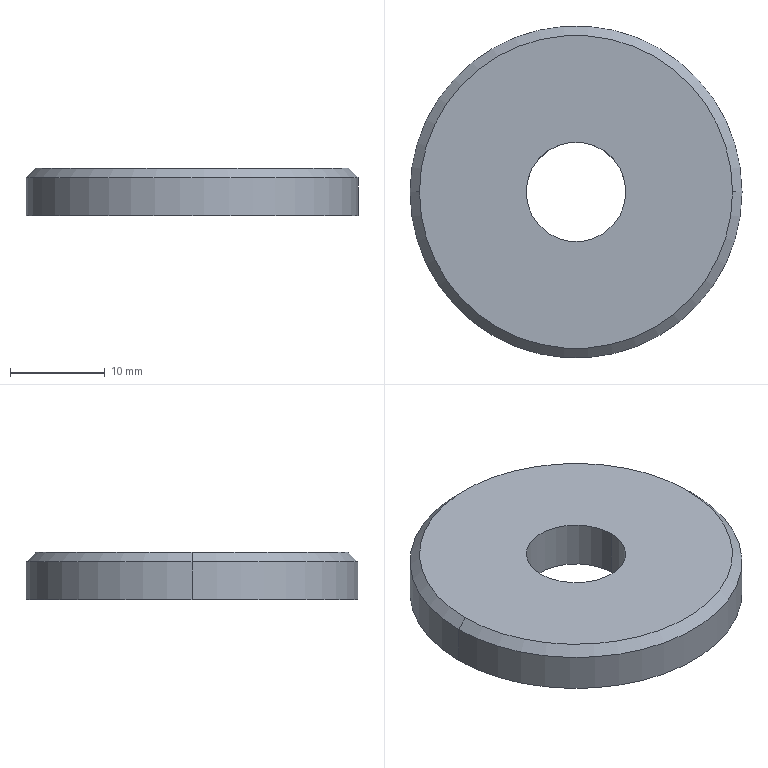Part | SolidWorks | features Chamfer 1, Extrusion 1 | 1 solid | 8 faces | box 35 x 35 x 5 mm | volume 4324 mm3 | cylinder 4 | cone 2 | plane 2 | commonest cylinder face diameters 10.5 x2 35 x2
STEP:
#1=CARTESIAN_POINT('',(16.5,0.,5.));
#2=VERTEX_POINT('',#1);
#3=CARTESIAN_POINT('',(-16.5,0.,5.));
#4=VERTEX_POINT('',#3);
#5=CARTESIAN_POINT('',(0.,0.,5.));
#6=DIRECTION('',(0.,0.,1.));
#7=DIRECTION('',(1.,0.,0.));
#8=AXIS2_PLACEMENT_3D('',#5,#6,#7);
#9=CIRCLE('',#8,16.5);
#10=EDGE_CURVE('',#2,#4,#9,.T.);
#11=ORIENTED_EDGE('',*,*,#10,.F.);
#12=CARTESIAN_POINT('',(17.5,0.,4.));
#13=VERTEX_POINT('',#12);
#14=CARTESIAN_POINT('',(16.5,0.,5.));
#15=DIRECTION('',(0.7071,0.,-0.7071));
#16=VECTOR('',#15,1000.);
#17=LINE('',#14,#16);
#18=EDGE_CURVE('',#2,#13,#17,.T.);
#19=ORIENTED_EDGE('',*,*,#18,.T.);
#20=CARTESIAN_POINT('',(-17.5,0.,4.));
#21=VERTEX_POINT('',#20);
#22=CARTESIAN_POINT('',(0.,0.,4.));
#23=DIRECTION('',(0.,0.,-1.));
#24=DIRECTION('',(1.,0.,0.));
#25=AXIS2_PLACEMENT_3D('',#22,#23,#24);
#26=CIRCLE('',#25,17.5);
#27=EDGE_CURVE('',#21,#13,#26,.T.);
#28=ORIENTED_EDGE('',*,*,#27,.F.);
#29=CARTESIAN_POINT('',(-16.5,0.,5.));
#30=DIRECTION('',(-0.7071,0.,-0.7071));
#31=VECTOR('',#30,1000.);
#32=LINE('',#29,#31);
#33=EDGE_CURVE('',#4,#21,#32,.T.);
#34=ORIENTED_EDGE('',*,*,#33,.F.);
#35=EDGE_LOOP('',(#11,#19,#28,#34));
#36=FACE_OUTER_BOUND('',#35,.T.);
#37=CARTESIAN_POINT('',(0.,0.,5.));
#38=DIRECTION('',(0.,0.,-1.));
#39=DIRECTION('',(-1.,0.,0.));
#40=AXIS2_PLACEMENT_3D('',#37,#38,#39);
#41=CONICAL_SURFACE('',#40,16.5,0.7854);
#42=ADVANCED_FACE('',(#36),#41,.T.);
#43=CARTESIAN_POINT('',(-5.25,0.,5.));
#44=VERTEX_POINT('',#43);
#45=CARTESIAN_POINT('',(5.25,0.,5.));
#46=VERTEX_POINT('',#45);
#47=CARTESIAN_POINT('',(0.,0.,5.));
#48=DIRECTION('',(0.,0.,1.));
#49=DIRECTION('',(1.,0.,0.));
#50=AXIS2_PLACEMENT_3D('',#47,#48,#49);
#51=CIRCLE('',#50,5.25);
#52=EDGE_CURVE('',#44,#46,#51,.T.);
#53=ORIENTED_EDGE('',*,*,#52,.T.);
#54=CARTESIAN_POINT('',(5.25,0.,0.));
#55=VERTEX_POINT('',#54);
#56=CARTESIAN_POINT('',(5.25,0.,5.));
#57=DIRECTION('',(0.,0.,-1.));
#58=VECTOR('',#57,1000.);
#59=LINE('',#56,#58);
#60=EDGE_CURVE('',#46,#55,#59,.T.);
#61=ORIENTED_EDGE('',*,*,#60,.T.);
#62=CARTESIAN_POINT('',(-5.25,0.,0.));
#63=VERTEX_POINT('',#62);
#64=CARTESIAN_POINT('',(0.,0.,0.));
#65=DIRECTION('',(0.,0.,1.));
#66=DIRECTION('',(1.,0.,0.));
#67=AXIS2_PLACEMENT_3D('',#64,#65,#66);
#68=CIRCLE('',#67,5.25);
#69=EDGE_CURVE('',#63,#55,#68,.T.);
#70=ORIENTED_EDGE('',*,*,#69,.F.);
#71=CARTESIAN_POINT('',(-5.25,0.,5.));
#72=DIRECTION('',(0.,0.,-1.));
#73=VECTOR('',#72,1000.);
#74=LINE('',#71,#73);
#75=EDGE_CURVE('',#44,#63,#74,.T.);
#76=ORIENTED_EDGE('',*,*,#75,.F.);
#77=EDGE_LOOP('',(#53,#61,#70,#76));
#78=FACE_OUTER_BOUND('',#77,.T.);
#79=CARTESIAN_POINT('',(0.,0.,5.));
#80=DIRECTION('',(0.,0.,-1.));
#81=DIRECTION('',(-1.,0.,0.));
#82=AXIS2_PLACEMENT_3D('',#79,#80,#81);
#83=CYLINDRICAL_SURFACE('',#82,5.25);
#84=ADVANCED_FACE('',(#78),#83,.F.);
#85=ORIENTED_EDGE('',*,*,#27,.T.);
#86=CARTESIAN_POINT('',(17.5,0.,0.));
#87=VERTEX_POINT('',#86);
#88=CARTESIAN_POINT('',(17.5,0.,5.));
#89=DIRECTION('',(0.,0.,-1.));
#90=VECTOR('',#89,1000.);
#91=LINE('',#88,#90);
#92=EDGE_CURVE('',#13,#87,#91,.T.);
#93=ORIENTED_EDGE('',*,*,#92,.T.);
#94=CARTESIAN_POINT('',(-17.5,0.,0.));
#95=VERTEX_POINT('',#94);
#96=CARTESIAN_POINT('',(0.,0.,0.));
#97=DIRECTION('',(0.,0.,1.));
#98=DIRECTION('',(1.,0.,0.));
#99=AXIS2_PLACEMENT_3D('',#96,#97,#98);
#100=CIRCLE('',#99,17.5);
#101=EDGE_CURVE('',#87,#95,#100,.T.);
#102=ORIENTED_EDGE('',*,*,#101,.T.);
#103=CARTESIAN_POINT('',(-17.5,0.,5.));
#104=DIRECTION('',(0.,0.,-1.));
#105=VECTOR('',#104,1000.);
#106=LINE('',#103,#105);
#107=EDGE_CURVE('',#21,#95,#106,.T.);
#108=ORIENTED_EDGE('',*,*,#107,.F.);
#109=EDGE_LOOP('',(#85,#93,#102,#108));
#110=FACE_OUTER_BOUND('',#109,.T.);
#111=CARTESIAN_POINT('',(0.,0.,5.));
#112=DIRECTION('',(0.,0.,-1.));
#113=DIRECTION('',(-1.,0.,0.));
#114=AXIS2_PLACEMENT_3D('',#111,#112,#113);
#115=CYLINDRICAL_SURFACE('',#114,17.5);
#116=ADVANCED_FACE('',(#110),#115,.T.);
#117=CARTESIAN_POINT('',(0.,0.,5.));
#118=DIRECTION('',(0.,0.,1.));
#119=DIRECTION('',(1.,0.,0.));
#120=AXIS2_PLACEMENT_3D('',#117,#118,#119);
#121=CIRCLE('',#120,16.5);
#122=EDGE_CURVE('',#4,#2,#121,.T.);
#123=ORIENTED_EDGE('',*,*,#122,.T.);
#124=ORIENTED_EDGE('',*,*,#10,.T.);
#125=EDGE_LOOP('',(#123,#124));
#126=FACE_OUTER_BOUND('',#125,.T.);
#127=ORIENTED_EDGE('',*,*,#52,.F.);
#128=CARTESIAN_POINT('',(0.,0.,5.));
#129=DIRECTION('',(0.,0.,1.));
#130=DIRECTION('',(1.,0.,0.));
#131=AXIS2_PLACEMENT_3D('',#128,#129,#130);
#132=CIRCLE('',#131,5.25);
#133=EDGE_CURVE('',#46,#44,#132,.T.);
#134=ORIENTED_EDGE('',*,*,#133,.F.);
#135=EDGE_LOOP('',(#127,#134));
#136=FACE_BOUND('',#135,.T.);
#137=CARTESIAN_POINT('',(0.,0.,5.));
#138=DIRECTION('',(0.,0.,1.));
#139=DIRECTION('',(1.,0.,0.));
#140=AXIS2_PLACEMENT_3D('',#137,#138,#139);
#141=PLANE('',#140);
#142=ADVANCED_FACE('',(#126,#136),#141,.T.);
#143=CARTESIAN_POINT('',(0.,0.,0.));
#144=DIRECTION('',(0.,0.,1.));
#145=DIRECTION('',(1.,0.,0.));
#146=AXIS2_PLACEMENT_3D('',#143,#144,#145);
#147=CIRCLE('',#146,17.5);
#148=EDGE_CURVE('',#95,#87,#147,.T.);
#149=ORIENTED_EDGE('',*,*,#148,.F.);
#150=ORIENTED_EDGE('',*,*,#101,.F.);
#151=EDGE_LOOP('',(#149,#150));
#152=FACE_OUTER_BOUND('',#151,.T.);
#153=ORIENTED_EDGE('',*,*,#69,.T.);
#154=CARTESIAN_POINT('',(0.,0.,0.));
#155=DIRECTION('',(0.,0.,1.));
#156=DIRECTION('',(1.,0.,0.));
#157=AXIS2_PLACEMENT_3D('',#154,#155,#156);
#158=CIRCLE('',#157,5.25);
#159=EDGE_CURVE('',#55,#63,#158,.T.);
#160=ORIENTED_EDGE('',*,*,#159,.T.);
#161=EDGE_LOOP('',(#153,#160));
#162=FACE_BOUND('',#161,.T.);
#163=CARTESIAN_POINT('',(0.,0.,0.));
#164=DIRECTION('',(0.,0.,1.));
#165=DIRECTION('',(1.,0.,0.));
#166=AXIS2_PLACEMENT_3D('',#163,#164,#165);
#167=PLANE('',#166);
#168=ADVANCED_FACE('',(#152,#162),#167,.F.);
#169=ORIENTED_EDGE('',*,*,#92,.F.);
#170=CARTESIAN_POINT('',(0.,0.,4.));
#171=DIRECTION('',(0.,0.,-1.));
#172=DIRECTION('',(1.,0.,0.));
#173=AXIS2_PLACEMENT_3D('',#170,#171,#172);
#174=CIRCLE('',#173,17.5);
#175=EDGE_CURVE('',#13,#21,#174,.T.);
#176=ORIENTED_EDGE('',*,*,#175,.T.);
#177=ORIENTED_EDGE('',*,*,#107,.T.);
#178=ORIENTED_EDGE('',*,*,#148,.T.);
#179=EDGE_LOOP('',(#169,#176,#177,#178));
#180=FACE_OUTER_BOUND('',#179,.T.);
#181=CARTESIAN_POINT('',(0.,0.,5.));
#182=DIRECTION('',(0.,0.,-1.));
#183=DIRECTION('',(-1.,0.,0.));
#184=AXIS2_PLACEMENT_3D('',#181,#182,#183);
#185=CYLINDRICAL_SURFACE('',#184,17.5);
#186=ADVANCED_FACE('',(#180),#185,.T.);
#187=ORIENTED_EDGE('',*,*,#60,.F.);
#188=ORIENTED_EDGE('',*,*,#133,.T.);
#189=ORIENTED_EDGE('',*,*,#75,.T.);
#190=ORIENTED_EDGE('',*,*,#159,.F.);
#191=EDGE_LOOP('',(#187,#188,#189,#190));
#192=FACE_OUTER_BOUND('',#191,.T.);
#193=CARTESIAN_POINT('',(0.,0.,5.));
#194=DIRECTION('',(0.,0.,-1.));
#195=DIRECTION('',(-1.,0.,0.));
#196=AXIS2_PLACEMENT_3D('',#193,#194,#195);
#197=CYLINDRICAL_SURFACE('',#196,5.25);
#198=ADVANCED_FACE('',(#192),#197,.F.);
#199=ORIENTED_EDGE('',*,*,#18,.F.);
#200=ORIENTED_EDGE('',*,*,#122,.F.);
#201=ORIENTED_EDGE('',*,*,#33,.T.);
#202=ORIENTED_EDGE('',*,*,#175,.F.);
#203=EDGE_LOOP('',(#199,#200,#201,#202));
#204=FACE_OUTER_BOUND('',#203,.T.);
#205=CARTESIAN_POINT('',(0.,0.,5.));
#206=DIRECTION('',(0.,0.,-1.));
#207=DIRECTION('',(-1.,0.,0.));
#208=AXIS2_PLACEMENT_3D('',#205,#206,#207);
#209=CONICAL_SURFACE('',#208,16.5,0.7854);
#210=ADVANCED_FACE('',(#204),#209,.T.);
#211=CLOSED_SHELL('',(#42,#84,#116,#142,#168,#186,#198,#210));
#212=MANIFOLD_SOLID_BREP('',#211);
#213=CARTESIAN_POINT('',(0.,0.,0.));
#214=DIRECTION('',(0.,0.,1.));
#215=DIRECTION('',(1.,0.,0.));
#216=AXIS2_PLACEMENT_3D('',#213,#214,#215);
#217=(LENGTH_UNIT()NAMED_UNIT(*)SI_UNIT(.MILLI.,.METRE.));
#218=UNCERTAINTY_MEASURE_WITH_UNIT(LENGTH_MEASURE(0.00001),#217,'','');
#219=(NAMED_UNIT(*)PLANE_ANGLE_UNIT()SI_UNIT($,.RADIAN.));
#220=(NAMED_UNIT(*)SI_UNIT($,.STERADIAN.)SOLID_ANGLE_UNIT());
#221=(GEOMETRIC_REPRESENTATION_CONTEXT(3)GLOBAL_UNCERTAINTY_ASSIGNED_CONTEXT((#218))GLOBAL_UNIT_ASSIGNED_CONTEXT((#217,#219,#220))REPRESENTATION_CONTEXT('',''));
#222=ADVANCED_BREP_SHAPE_REPRESENTATION('',(#212,#216),#221);